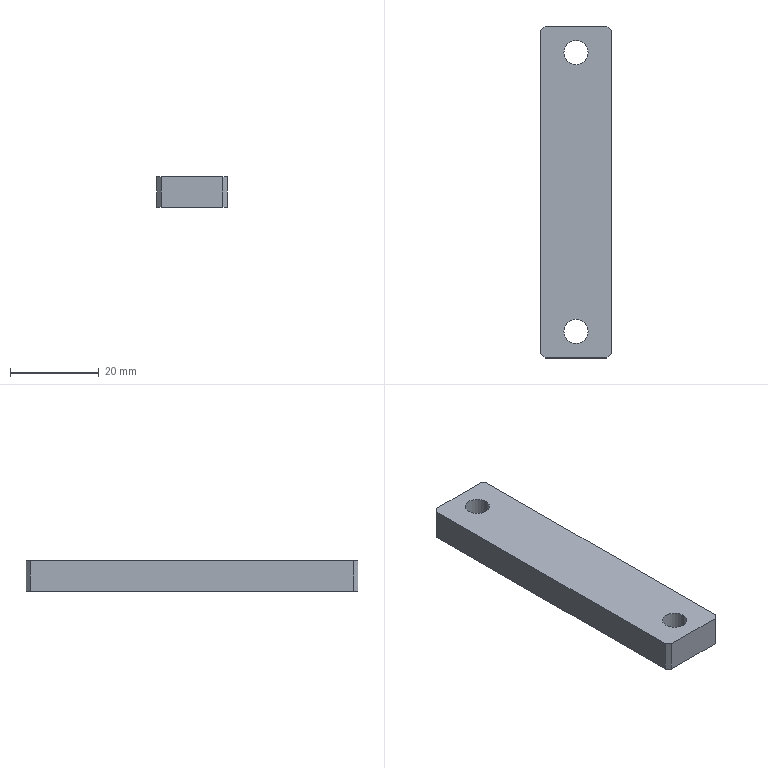Part | SolidWorks | features Chamfer 1, Extrusion 1, HoleWzd 1 | 1 solid | 14 faces | box 16 x 75 x 7 mm | volume 8053 mm3 | plane 10 | cylinder 4 | commonest cylinder face diameters 5.5 x4
STEP:
#1=CARTESIAN_POINT('',(-2.75,31.5,0.));
#2=VERTEX_POINT('',#1);
#3=CARTESIAN_POINT('',(2.75,31.5,0.));
#4=VERTEX_POINT('',#3);
#5=CARTESIAN_POINT('',(0.,31.5,0.));
#6=DIRECTION('',(0.,0.,1.));
#7=DIRECTION('',(1.,0.,0.));
#8=AXIS2_PLACEMENT_3D('',#5,#6,#7);
#9=CIRCLE('',#8,2.75);
#10=EDGE_CURVE('',#2,#4,#9,.T.);
#11=ORIENTED_EDGE('',*,*,#10,.F.);
#12=CARTESIAN_POINT('',(-2.75,31.5,7.));
#13=VERTEX_POINT('',#12);
#14=CARTESIAN_POINT('',(-2.75,31.5,7.));
#15=DIRECTION('',(0.,0.,1.));
#16=VECTOR('',#15,1000.);
#17=LINE('',#14,#16);
#18=EDGE_CURVE('',#2,#13,#17,.T.);
#19=ORIENTED_EDGE('',*,*,#18,.T.);
#20=CARTESIAN_POINT('',(2.75,31.5,7.));
#21=VERTEX_POINT('',#20);
#22=CARTESIAN_POINT('',(0.,31.5,7.));
#23=DIRECTION('',(0.,0.,1.));
#24=DIRECTION('',(1.,0.,0.));
#25=AXIS2_PLACEMENT_3D('',#22,#23,#24);
#26=CIRCLE('',#25,2.75);
#27=EDGE_CURVE('',#13,#21,#26,.T.);
#28=ORIENTED_EDGE('',*,*,#27,.T.);
#29=CARTESIAN_POINT('',(2.75,31.5,7.));
#30=DIRECTION('',(0.,0.,1.));
#31=VECTOR('',#30,1000.);
#32=LINE('',#29,#31);
#33=EDGE_CURVE('',#4,#21,#32,.T.);
#34=ORIENTED_EDGE('',*,*,#33,.F.);
#35=EDGE_LOOP('',(#11,#19,#28,#34));
#36=FACE_OUTER_BOUND('',#35,.T.);
#37=CARTESIAN_POINT('',(0.,31.5,7.));
#38=DIRECTION('',(0.,0.,1.));
#39=DIRECTION('',(1.,0.,0.));
#40=AXIS2_PLACEMENT_3D('',#37,#38,#39);
#41=CYLINDRICAL_SURFACE('',#40,2.75);
#42=ADVANCED_FACE('',(#36),#41,.F.);
#43=CARTESIAN_POINT('',(-2.75,-31.5,0.));
#44=VERTEX_POINT('',#43);
#45=CARTESIAN_POINT('',(2.75,-31.5,0.));
#46=VERTEX_POINT('',#45);
#47=CARTESIAN_POINT('',(0.,-31.5,0.));
#48=DIRECTION('',(0.,0.,1.));
#49=DIRECTION('',(1.,0.,0.));
#50=AXIS2_PLACEMENT_3D('',#47,#48,#49);
#51=CIRCLE('',#50,2.75);
#52=EDGE_CURVE('',#44,#46,#51,.T.);
#53=ORIENTED_EDGE('',*,*,#52,.F.);
#54=CARTESIAN_POINT('',(-2.75,-31.5,7.));
#55=VERTEX_POINT('',#54);
#56=CARTESIAN_POINT('',(-2.75,-31.5,7.));
#57=DIRECTION('',(0.,0.,1.));
#58=VECTOR('',#57,1000.);
#59=LINE('',#56,#58);
#60=EDGE_CURVE('',#44,#55,#59,.T.);
#61=ORIENTED_EDGE('',*,*,#60,.T.);
#62=CARTESIAN_POINT('',(2.75,-31.5,7.));
#63=VERTEX_POINT('',#62);
#64=CARTESIAN_POINT('',(0.,-31.5,7.));
#65=DIRECTION('',(0.,0.,1.));
#66=DIRECTION('',(1.,0.,0.));
#67=AXIS2_PLACEMENT_3D('',#64,#65,#66);
#68=CIRCLE('',#67,2.75);
#69=EDGE_CURVE('',#55,#63,#68,.T.);
#70=ORIENTED_EDGE('',*,*,#69,.T.);
#71=CARTESIAN_POINT('',(2.75,-31.5,7.));
#72=DIRECTION('',(0.,0.,1.));
#73=VECTOR('',#72,1000.);
#74=LINE('',#71,#73);
#75=EDGE_CURVE('',#46,#63,#74,.T.);
#76=ORIENTED_EDGE('',*,*,#75,.F.);
#77=EDGE_LOOP('',(#53,#61,#70,#76));
#78=FACE_OUTER_BOUND('',#77,.T.);
#79=CARTESIAN_POINT('',(0.,-31.5,7.));
#80=DIRECTION('',(0.,0.,1.));
#81=DIRECTION('',(1.,0.,0.));
#82=AXIS2_PLACEMENT_3D('',#79,#80,#81);
#83=CYLINDRICAL_SURFACE('',#82,2.75);
#84=ADVANCED_FACE('',(#78),#83,.F.);
#85=CARTESIAN_POINT('',(8.,-36.5,0.));
#86=VERTEX_POINT('',#85);
#87=CARTESIAN_POINT('',(8.,36.5,0.));
#88=VERTEX_POINT('',#87);
#89=CARTESIAN_POINT('',(8.,37.5,0.));
#90=DIRECTION('',(0.,1.,0.));
#91=VECTOR('',#90,1000.);
#92=LINE('',#89,#91);
#93=EDGE_CURVE('',#86,#88,#92,.T.);
#94=ORIENTED_EDGE('',*,*,#93,.T.);
#95=CARTESIAN_POINT('',(8.,36.5,7.));
#96=VERTEX_POINT('',#95);
#97=CARTESIAN_POINT('',(8.,36.5,7.));
#98=DIRECTION('',(0.,0.,1.));
#99=VECTOR('',#98,1000.);
#100=LINE('',#97,#99);
#101=EDGE_CURVE('',#88,#96,#100,.T.);
#102=ORIENTED_EDGE('',*,*,#101,.T.);
#103=CARTESIAN_POINT('',(8.,-36.5,7.));
#104=VERTEX_POINT('',#103);
#105=CARTESIAN_POINT('',(8.,37.5,7.));
#106=DIRECTION('',(0.,1.,0.));
#107=VECTOR('',#106,1000.);
#108=LINE('',#105,#107);
#109=EDGE_CURVE('',#104,#96,#108,.T.);
#110=ORIENTED_EDGE('',*,*,#109,.F.);
#111=CARTESIAN_POINT('',(8.,-36.5,7.));
#112=DIRECTION('',(0.,0.,-1.));
#113=VECTOR('',#112,1000.);
#114=LINE('',#111,#113);
#115=EDGE_CURVE('',#104,#86,#114,.T.);
#116=ORIENTED_EDGE('',*,*,#115,.T.);
#117=EDGE_LOOP('',(#94,#102,#110,#116));
#118=FACE_OUTER_BOUND('',#117,.T.);
#119=CARTESIAN_POINT('',(8.,37.5,7.));
#120=DIRECTION('',(-1.,0.,0.));
#121=DIRECTION('',(0.,-1.,0.));
#122=AXIS2_PLACEMENT_3D('',#119,#120,#121);
#123=PLANE('',#122);
#124=ADVANCED_FACE('',(#118),#123,.F.);
#125=CARTESIAN_POINT('',(7.,37.5,0.));
#126=VERTEX_POINT('',#125);
#127=CARTESIAN_POINT('',(-7.,37.5,0.));
#128=VERTEX_POINT('',#127);
#129=CARTESIAN_POINT('',(-8.,37.5,0.));
#130=DIRECTION('',(-1.,0.,0.));
#131=VECTOR('',#130,1000.);
#132=LINE('',#129,#131);
#133=EDGE_CURVE('',#126,#128,#132,.T.);
#134=ORIENTED_EDGE('',*,*,#133,.T.);
#135=CARTESIAN_POINT('',(-7.,37.5,7.));
#136=VERTEX_POINT('',#135);
#137=CARTESIAN_POINT('',(-7.,37.5,7.));
#138=DIRECTION('',(0.,0.,1.));
#139=VECTOR('',#138,1000.);
#140=LINE('',#137,#139);
#141=EDGE_CURVE('',#128,#136,#140,.T.);
#142=ORIENTED_EDGE('',*,*,#141,.T.);
#143=CARTESIAN_POINT('',(7.,37.5,7.));
#144=VERTEX_POINT('',#143);
#145=CARTESIAN_POINT('',(-8.,37.5,7.));
#146=DIRECTION('',(-1.,0.,0.));
#147=VECTOR('',#146,1000.);
#148=LINE('',#145,#147);
#149=EDGE_CURVE('',#144,#136,#148,.T.);
#150=ORIENTED_EDGE('',*,*,#149,.F.);
#151=CARTESIAN_POINT('',(7.,37.5,7.));
#152=DIRECTION('',(0.,0.,-1.));
#153=VECTOR('',#152,1000.);
#154=LINE('',#151,#153);
#155=EDGE_CURVE('',#144,#126,#154,.T.);
#156=ORIENTED_EDGE('',*,*,#155,.T.);
#157=EDGE_LOOP('',(#134,#142,#150,#156));
#158=FACE_OUTER_BOUND('',#157,.T.);
#159=CARTESIAN_POINT('',(-8.,37.5,7.));
#160=DIRECTION('',(0.,-1.,0.));
#161=DIRECTION('',(0.,0.,-1.));
#162=AXIS2_PLACEMENT_3D('',#159,#160,#161);
#163=PLANE('',#162);
#164=ADVANCED_FACE('',(#158),#163,.F.);
#165=CARTESIAN_POINT('',(-8.,36.5,0.));
#166=VERTEX_POINT('',#165);
#167=CARTESIAN_POINT('',(-8.,-36.5,0.));
#168=VERTEX_POINT('',#167);
#169=CARTESIAN_POINT('',(-8.,37.5,0.));
#170=DIRECTION('',(0.,-1.,0.));
#171=VECTOR('',#170,1000.);
#172=LINE('',#169,#171);
#173=EDGE_CURVE('',#166,#168,#172,.T.);
#174=ORIENTED_EDGE('',*,*,#173,.T.);
#175=CARTESIAN_POINT('',(-8.,-36.5,7.));
#176=VERTEX_POINT('',#175);
#177=CARTESIAN_POINT('',(-8.,-36.5,7.));
#178=DIRECTION('',(0.,0.,1.));
#179=VECTOR('',#178,1000.);
#180=LINE('',#177,#179);
#181=EDGE_CURVE('',#168,#176,#180,.T.);
#182=ORIENTED_EDGE('',*,*,#181,.T.);
#183=CARTESIAN_POINT('',(-8.,36.5,7.));
#184=VERTEX_POINT('',#183);
#185=CARTESIAN_POINT('',(-8.,37.5,7.));
#186=DIRECTION('',(0.,-1.,0.));
#187=VECTOR('',#186,1000.);
#188=LINE('',#185,#187);
#189=EDGE_CURVE('',#184,#176,#188,.T.);
#190=ORIENTED_EDGE('',*,*,#189,.F.);
#191=CARTESIAN_POINT('',(-8.,36.5,7.));
#192=DIRECTION('',(0.,0.,-1.));
#193=VECTOR('',#192,1000.);
#194=LINE('',#191,#193);
#195=EDGE_CURVE('',#184,#166,#194,.T.);
#196=ORIENTED_EDGE('',*,*,#195,.T.);
#197=EDGE_LOOP('',(#174,#182,#190,#196));
#198=FACE_OUTER_BOUND('',#197,.T.);
#199=CARTESIAN_POINT('',(-8.,37.5,7.));
#200=DIRECTION('',(1.,0.,0.));
#201=DIRECTION('',(0.,1.,0.));
#202=AXIS2_PLACEMENT_3D('',#199,#200,#201);
#203=PLANE('',#202);
#204=ADVANCED_FACE('',(#198),#203,.F.);
#205=CARTESIAN_POINT('',(-7.,-37.5,7.));
#206=VERTEX_POINT('',#205);
#207=CARTESIAN_POINT('',(7.,-37.5,7.));
#208=VERTEX_POINT('',#207);
#209=CARTESIAN_POINT('',(-8.,-37.5,7.));
#210=DIRECTION('',(1.,0.,0.));
#211=VECTOR('',#210,1000.);
#212=LINE('',#209,#211);
#213=EDGE_CURVE('',#206,#208,#212,.T.);
#214=ORIENTED_EDGE('',*,*,#213,.F.);
#215=CARTESIAN_POINT('',(-7.,-37.5,0.));
#216=VERTEX_POINT('',#215);
#217=CARTESIAN_POINT('',(-7.,-37.5,7.));
#218=DIRECTION('',(0.,0.,-1.));
#219=VECTOR('',#218,1000.);
#220=LINE('',#217,#219);
#221=EDGE_CURVE('',#206,#216,#220,.T.);
#222=ORIENTED_EDGE('',*,*,#221,.T.);
#223=CARTESIAN_POINT('',(7.,-37.5,0.));
#224=VERTEX_POINT('',#223);
#225=CARTESIAN_POINT('',(-8.,-37.5,0.));
#226=DIRECTION('',(1.,0.,0.));
#227=VECTOR('',#226,1000.);
#228=LINE('',#225,#227);
#229=EDGE_CURVE('',#216,#224,#228,.T.);
#230=ORIENTED_EDGE('',*,*,#229,.T.);
#231=CARTESIAN_POINT('',(7.,-37.5,7.));
#232=DIRECTION('',(0.,0.,1.));
#233=VECTOR('',#232,1000.);
#234=LINE('',#231,#233);
#235=EDGE_CURVE('',#224,#208,#234,.T.);
#236=ORIENTED_EDGE('',*,*,#235,.T.);
#237=EDGE_LOOP('',(#214,#222,#230,#236));
#238=FACE_OUTER_BOUND('',#237,.T.);
#239=CARTESIAN_POINT('',(-8.,-37.5,7.));
#240=DIRECTION('',(0.,1.,0.));
#241=DIRECTION('',(0.,0.,1.));
#242=AXIS2_PLACEMENT_3D('',#239,#240,#241);
#243=PLANE('',#242);
#244=ADVANCED_FACE('',(#238),#243,.F.);
#245=CARTESIAN_POINT('',(0.,31.5,7.));
#246=DIRECTION('',(0.,0.,1.));
#247=DIRECTION('',(1.,0.,0.));
#248=AXIS2_PLACEMENT_3D('',#245,#246,#247);
#249=CIRCLE('',#248,2.75);
#250=EDGE_CURVE('',#21,#13,#249,.T.);
#251=ORIENTED_EDGE('',*,*,#250,.F.);
#252=ORIENTED_EDGE('',*,*,#27,.F.);
#253=EDGE_LOOP('',(#251,#252));
#254=FACE_BOUND('',#253,.T.);
#255=CARTESIAN_POINT('',(0.,-31.5,7.));
#256=DIRECTION('',(0.,0.,1.));
#257=DIRECTION('',(1.,0.,0.));
#258=AXIS2_PLACEMENT_3D('',#255,#256,#257);
#259=CIRCLE('',#258,2.75);
#260=EDGE_CURVE('',#63,#55,#259,.T.);
#261=ORIENTED_EDGE('',*,*,#260,.F.);
#262=ORIENTED_EDGE('',*,*,#69,.F.);
#263=EDGE_LOOP('',(#261,#262));
#264=FACE_BOUND('',#263,.T.);
#265=ORIENTED_EDGE('',*,*,#189,.T.);
#266=CARTESIAN_POINT('',(-22.25,-22.25,7.));
#267=DIRECTION('',(0.7071,-0.7071,0.));
#268=VECTOR('',#267,1000.);
#269=LINE('',#266,#268);
#270=EDGE_CURVE('',#176,#206,#269,.T.);
#271=ORIENTED_EDGE('',*,*,#270,.T.);
#272=ORIENTED_EDGE('',*,*,#213,.T.);
#273=CARTESIAN_POINT('',(22.25,-22.25,7.));
#274=DIRECTION('',(0.7071,0.7071,0.));
#275=VECTOR('',#274,1000.);
#276=LINE('',#273,#275);
#277=EDGE_CURVE('',#208,#104,#276,.T.);
#278=ORIENTED_EDGE('',*,*,#277,.T.);
#279=ORIENTED_EDGE('',*,*,#109,.T.);
#280=CARTESIAN_POINT('',(22.25,22.25,7.));
#281=DIRECTION('',(-0.7071,0.7071,0.));
#282=VECTOR('',#281,1000.);
#283=LINE('',#280,#282);
#284=EDGE_CURVE('',#96,#144,#283,.T.);
#285=ORIENTED_EDGE('',*,*,#284,.T.);
#286=ORIENTED_EDGE('',*,*,#149,.T.);
#287=CARTESIAN_POINT('',(-22.25,22.25,7.));
#288=DIRECTION('',(-0.7071,-0.7071,0.));
#289=VECTOR('',#288,1000.);
#290=LINE('',#287,#289);
#291=EDGE_CURVE('',#136,#184,#290,.T.);
#292=ORIENTED_EDGE('',*,*,#291,.T.);
#293=EDGE_LOOP('',(#265,#271,#272,#278,#279,#285,#286,#292));
#294=FACE_OUTER_BOUND('',#293,.T.);
#295=CARTESIAN_POINT('',(0.,0.,7.));
#296=DIRECTION('',(0.,0.,1.));
#297=DIRECTION('',(1.,0.,0.));
#298=AXIS2_PLACEMENT_3D('',#295,#296,#297);
#299=PLANE('',#298);
#300=ADVANCED_FACE('',(#254,#264,#294),#299,.T.);
#301=CARTESIAN_POINT('',(0.,31.5,0.));
#302=DIRECTION('',(0.,0.,1.));
#303=DIRECTION('',(1.,0.,0.));
#304=AXIS2_PLACEMENT_3D('',#301,#302,#303);
#305=CIRCLE('',#304,2.75);
#306=EDGE_CURVE('',#4,#2,#305,.T.);
#307=ORIENTED_EDGE('',*,*,#306,.T.);
#308=ORIENTED_EDGE('',*,*,#10,.T.);
#309=EDGE_LOOP('',(#307,#308));
#310=FACE_BOUND('',#309,.T.);
#311=CARTESIAN_POINT('',(0.,-31.5,0.));
#312=DIRECTION('',(0.,0.,1.));
#313=DIRECTION('',(1.,0.,0.));
#314=AXIS2_PLACEMENT_3D('',#311,#312,#313);
#315=CIRCLE('',#314,2.75);
#316=EDGE_CURVE('',#46,#44,#315,.T.);
#317=ORIENTED_EDGE('',*,*,#316,.T.);
#318=ORIENTED_EDGE('',*,*,#52,.T.);
#319=EDGE_LOOP('',(#317,#318));
#320=FACE_BOUND('',#319,.T.);
#321=ORIENTED_EDGE('',*,*,#229,.F.);
#322=CARTESIAN_POINT('',(-7.,-37.5,0.));
#323=DIRECTION('',(-0.7071,0.7071,0.));
#324=VECTOR('',#323,1000.);
#325=LINE('',#322,#324);
#326=EDGE_CURVE('',#216,#168,#325,.T.);
#327=ORIENTED_EDGE('',*,*,#326,.T.);
#328=ORIENTED_EDGE('',*,*,#173,.F.);
#329=CARTESIAN_POINT('',(-8.,36.5,0.));
#330=DIRECTION('',(0.7071,0.7071,0.));
#331=VECTOR('',#330,1000.);
#332=LINE('',#329,#331);
#333=EDGE_CURVE('',#166,#128,#332,.T.);
#334=ORIENTED_EDGE('',*,*,#333,.T.);
#335=ORIENTED_EDGE('',*,*,#133,.F.);
#336=CARTESIAN_POINT('',(7.,37.5,0.));
#337=DIRECTION('',(0.7071,-0.7071,0.));
#338=VECTOR('',#337,1000.);
#339=LINE('',#336,#338);
#340=EDGE_CURVE('',#126,#88,#339,.T.);
#341=ORIENTED_EDGE('',*,*,#340,.T.);
#342=ORIENTED_EDGE('',*,*,#93,.F.);
#343=CARTESIAN_POINT('',(8.,-36.5,0.));
#344=DIRECTION('',(-0.7071,-0.7071,0.));
#345=VECTOR('',#344,1000.);
#346=LINE('',#343,#345);
#347=EDGE_CURVE('',#86,#224,#346,.T.);
#348=ORIENTED_EDGE('',*,*,#347,.T.);
#349=EDGE_LOOP('',(#321,#327,#328,#334,#335,#341,#342,#348));
#350=FACE_OUTER_BOUND('',#349,.T.);
#351=CARTESIAN_POINT('',(0.,0.,0.));
#352=DIRECTION('',(0.,0.,1.));
#353=DIRECTION('',(1.,0.,0.));
#354=AXIS2_PLACEMENT_3D('',#351,#352,#353);
#355=PLANE('',#354);
#356=ADVANCED_FACE('',(#310,#320,#350),#355,.F.);
#357=ORIENTED_EDGE('',*,*,#270,.F.);
#358=ORIENTED_EDGE('',*,*,#181,.F.);
#359=ORIENTED_EDGE('',*,*,#326,.F.);
#360=ORIENTED_EDGE('',*,*,#221,.F.);
#361=EDGE_LOOP('',(#357,#358,#359,#360));
#362=FACE_OUTER_BOUND('',#361,.T.);
#363=CARTESIAN_POINT('',(-7.,-37.5,7.));
#364=DIRECTION('',(0.7071,0.7071,0.));
#365=DIRECTION('',(0.,0.,-1.));
#366=AXIS2_PLACEMENT_3D('',#363,#364,#365);
#367=PLANE('',#366);
#368=ADVANCED_FACE('',(#362),#367,.F.);
#369=ORIENTED_EDGE('',*,*,#291,.F.);
#370=ORIENTED_EDGE('',*,*,#141,.F.);
#371=ORIENTED_EDGE('',*,*,#333,.F.);
#372=ORIENTED_EDGE('',*,*,#195,.F.);
#373=EDGE_LOOP('',(#369,#370,#371,#372));
#374=FACE_OUTER_BOUND('',#373,.T.);
#375=CARTESIAN_POINT('',(-8.,36.5,7.));
#376=DIRECTION('',(0.7071,-0.7071,0.));
#377=DIRECTION('',(0.,0.,-1.));
#378=AXIS2_PLACEMENT_3D('',#375,#376,#377);
#379=PLANE('',#378);
#380=ADVANCED_FACE('',(#374),#379,.F.);
#381=ORIENTED_EDGE('',*,*,#284,.F.);
#382=ORIENTED_EDGE('',*,*,#101,.F.);
#383=ORIENTED_EDGE('',*,*,#340,.F.);
#384=ORIENTED_EDGE('',*,*,#155,.F.);
#385=EDGE_LOOP('',(#381,#382,#383,#384));
#386=FACE_OUTER_BOUND('',#385,.T.);
#387=CARTESIAN_POINT('',(7.,37.5,7.));
#388=DIRECTION('',(-0.7071,-0.7071,0.));
#389=DIRECTION('',(0.,0.,-1.));
#390=AXIS2_PLACEMENT_3D('',#387,#388,#389);
#391=PLANE('',#390);
#392=ADVANCED_FACE('',(#386),#391,.F.);
#393=ORIENTED_EDGE('',*,*,#277,.F.);
#394=ORIENTED_EDGE('',*,*,#235,.F.);
#395=ORIENTED_EDGE('',*,*,#347,.F.);
#396=ORIENTED_EDGE('',*,*,#115,.F.);
#397=EDGE_LOOP('',(#393,#394,#395,#396));
#398=FACE_OUTER_BOUND('',#397,.T.);
#399=CARTESIAN_POINT('',(8.,-36.5,7.));
#400=DIRECTION('',(-0.7071,0.7071,0.));
#401=DIRECTION('',(0.,0.,-1.));
#402=AXIS2_PLACEMENT_3D('',#399,#400,#401);
#403=PLANE('',#402);
#404=ADVANCED_FACE('',(#398),#403,.F.);
#405=ORIENTED_EDGE('',*,*,#60,.F.);
#406=ORIENTED_EDGE('',*,*,#316,.F.);
#407=ORIENTED_EDGE('',*,*,#75,.T.);
#408=ORIENTED_EDGE('',*,*,#260,.T.);
#409=EDGE_LOOP('',(#405,#406,#407,#408));
#410=FACE_OUTER_BOUND('',#409,.T.);
#411=CARTESIAN_POINT('',(0.,-31.5,7.));
#412=DIRECTION('',(0.,0.,1.));
#413=DIRECTION('',(1.,0.,0.));
#414=AXIS2_PLACEMENT_3D('',#411,#412,#413);
#415=CYLINDRICAL_SURFACE('',#414,2.75);
#416=ADVANCED_FACE('',(#410),#415,.F.);
#417=ORIENTED_EDGE('',*,*,#18,.F.);
#418=ORIENTED_EDGE('',*,*,#306,.F.);
#419=ORIENTED_EDGE('',*,*,#33,.T.);
#420=ORIENTED_EDGE('',*,*,#250,.T.);
#421=EDGE_LOOP('',(#417,#418,#419,#420));
#422=FACE_OUTER_BOUND('',#421,.T.);
#423=CARTESIAN_POINT('',(0.,31.5,7.));
#424=DIRECTION('',(0.,0.,1.));
#425=DIRECTION('',(1.,0.,0.));
#426=AXIS2_PLACEMENT_3D('',#423,#424,#425);
#427=CYLINDRICAL_SURFACE('',#426,2.75);
#428=ADVANCED_FACE('',(#422),#427,.F.);
#429=CLOSED_SHELL('',(#42,#84,#124,#164,#204,#244,#300,#356,#368,#380,#392,#404,#416,#428));
#430=MANIFOLD_SOLID_BREP('',#429);
#431=CARTESIAN_POINT('',(0.,0.,0.));
#432=DIRECTION('',(0.,0.,1.));
#433=DIRECTION('',(1.,0.,0.));
#434=AXIS2_PLACEMENT_3D('',#431,#432,#433);
#435=(LENGTH_UNIT()NAMED_UNIT(*)SI_UNIT(.MILLI.,.METRE.));
#436=UNCERTAINTY_MEASURE_WITH_UNIT(LENGTH_MEASURE(0.00001),#435,'','');
#437=(NAMED_UNIT(*)PLANE_ANGLE_UNIT()SI_UNIT($,.RADIAN.));
#438=(NAMED_UNIT(*)SI_UNIT($,.STERADIAN.)SOLID_ANGLE_UNIT());
#439=(GEOMETRIC_REPRESENTATION_CONTEXT(3)GLOBAL_UNCERTAINTY_ASSIGNED_CONTEXT((#436))GLOBAL_UNIT_ASSIGNED_CONTEXT((#435,#437,#438))REPRESENTATION_CONTEXT('',''));
#440=ADVANCED_BREP_SHAPE_REPRESENTATION('',(#430,#434),#439);